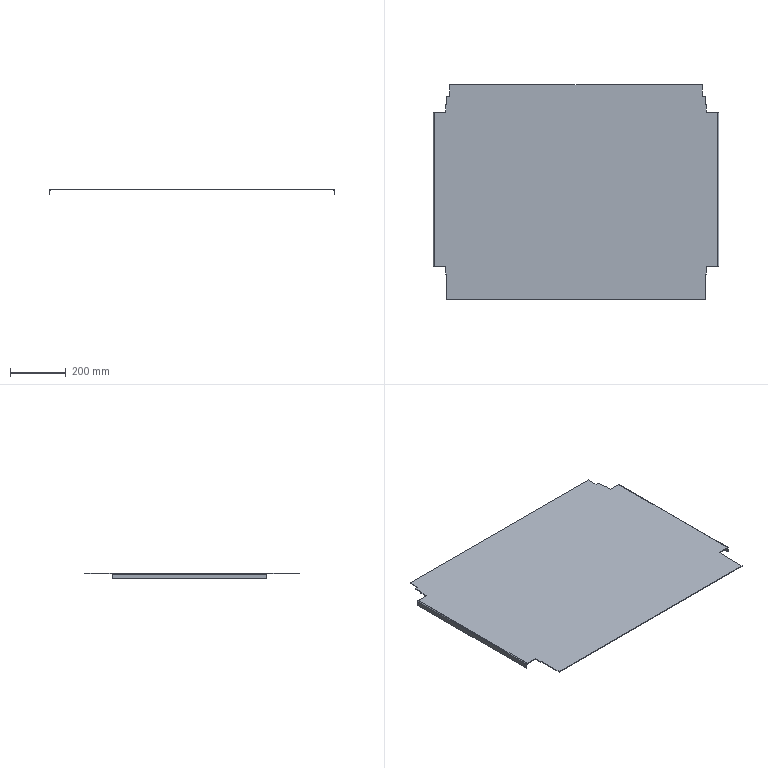Part | SolidWorks | features BaseBody 1 | 1 solid | 42 faces | box 1023 x 767.4 x 20 mm | volume 1955207 mm3 | plane 38 | cylinder 4 | commonest cylinder face diameters 2 x2 7 x2
STEP:
#1=CARTESIAN_POINT('',(509.,285.7,-20.));
#2=VERTEX_POINT('',#1);
#3=CARTESIAN_POINT('',(509.,-266.55,-20.));
#4=VERTEX_POINT('',#3);
#5=CARTESIAN_POINT('',(509.,0.,-20.));
#6=DIRECTION('',(0.,-1.,0.));
#7=VECTOR('',#6,1000.);
#8=LINE('',#5,#7);
#9=EDGE_CURVE('',#2,#4,#8,.T.);
#10=ORIENTED_EDGE('',*,*,#9,.F.);
#11=CARTESIAN_POINT('',(511.5,285.7,-20.));
#12=VERTEX_POINT('',#11);
#13=CARTESIAN_POINT('',(511.5,285.7,-20.));
#14=DIRECTION('',(-1.,0.,0.));
#15=VECTOR('',#14,1000.);
#16=LINE('',#13,#15);
#17=EDGE_CURVE('',#12,#2,#16,.T.);
#18=ORIENTED_EDGE('',*,*,#17,.F.);
#19=CARTESIAN_POINT('',(511.5,-266.55,-20.));
#20=VERTEX_POINT('',#19);
#21=CARTESIAN_POINT('',(511.5,-266.55,-20.));
#22=DIRECTION('',(0.,-1.,0.));
#23=VECTOR('',#22,1000.);
#24=LINE('',#21,#23);
#25=EDGE_CURVE('',#12,#20,#24,.T.);
#26=ORIENTED_EDGE('',*,*,#25,.T.);
#27=CARTESIAN_POINT('',(511.5,-266.55,-20.));
#28=DIRECTION('',(-1.,0.,0.));
#29=VECTOR('',#28,1000.);
#30=LINE('',#27,#29);
#31=EDGE_CURVE('',#20,#4,#30,.T.);
#32=ORIENTED_EDGE('',*,*,#31,.T.);
#33=EDGE_LOOP('',(#10,#18,#26,#32));
#34=FACE_OUTER_BOUND('',#33,.T.);
#35=CARTESIAN_POINT('',(511.5,-266.55,-20.));
#36=DIRECTION('',(0.,0.,-1.));
#37=DIRECTION('',(0.,-1.,0.));
#38=AXIS2_PLACEMENT_3D('',#35,#36,#37);
#39=PLANE('',#38);
#40=ADVANCED_FACE('',(#34),#39,.T.);
#41=CARTESIAN_POINT('',(509.,285.7,-3.5));
#42=VERTEX_POINT('',#41);
#43=CARTESIAN_POINT('',(509.,-266.55,-3.5));
#44=VERTEX_POINT('',#43);
#45=CARTESIAN_POINT('',(509.,285.7,-3.5));
#46=DIRECTION('',(0.,-1.,0.));
#47=VECTOR('',#46,1000.);
#48=LINE('',#45,#47);
#49=EDGE_CURVE('',#42,#44,#48,.T.);
#50=ORIENTED_EDGE('',*,*,#49,.F.);
#51=CARTESIAN_POINT('',(509.,285.7,0.));
#52=DIRECTION('',(0.,0.,-1.));
#53=VECTOR('',#52,1000.);
#54=LINE('',#51,#53);
#55=EDGE_CURVE('',#42,#2,#54,.T.);
#56=ORIENTED_EDGE('',*,*,#55,.T.);
#57=ORIENTED_EDGE('',*,*,#9,.T.);
#58=CARTESIAN_POINT('',(509.,-266.55,0.));
#59=DIRECTION('',(0.,0.,1.));
#60=VECTOR('',#59,1000.);
#61=LINE('',#58,#60);
#62=EDGE_CURVE('',#4,#44,#61,.T.);
#63=ORIENTED_EDGE('',*,*,#62,.T.);
#64=EDGE_LOOP('',(#50,#56,#57,#63));
#65=FACE_OUTER_BOUND('',#64,.T.);
#66=CARTESIAN_POINT('',(509.,0.,0.));
#67=DIRECTION('',(1.,0.,0.));
#68=DIRECTION('',(0.,0.,1.));
#69=AXIS2_PLACEMENT_3D('',#66,#67,#68);
#70=PLANE('',#69);
#71=ADVANCED_FACE('',(#65),#70,.F.);
#72=CARTESIAN_POINT('',(511.5,285.7,-3.5));
#73=VERTEX_POINT('',#72);
#74=CARTESIAN_POINT('',(511.5,285.7,-20.));
#75=DIRECTION('',(0.,0.,-1.));
#76=VECTOR('',#75,1000.);
#77=LINE('',#74,#76);
#78=EDGE_CURVE('',#73,#12,#77,.T.);
#79=ORIENTED_EDGE('',*,*,#78,.F.);
#80=CARTESIAN_POINT('',(511.5,-266.55,-3.5));
#81=VERTEX_POINT('',#80);
#82=CARTESIAN_POINT('',(511.5,0.,-3.5));
#83=DIRECTION('',(0.,-1.,0.));
#84=VECTOR('',#83,1000.);
#85=LINE('',#82,#84);
#86=EDGE_CURVE('',#73,#81,#85,.T.);
#87=ORIENTED_EDGE('',*,*,#86,.T.);
#88=CARTESIAN_POINT('',(511.5,-266.55,-2.5));
#89=DIRECTION('',(0.,0.,1.));
#90=VECTOR('',#89,1000.);
#91=LINE('',#88,#90);
#92=EDGE_CURVE('',#20,#81,#91,.T.);
#93=ORIENTED_EDGE('',*,*,#92,.F.);
#94=ORIENTED_EDGE('',*,*,#25,.F.);
#95=EDGE_LOOP('',(#79,#87,#93,#94));
#96=FACE_OUTER_BOUND('',#95,.T.);
#97=CARTESIAN_POINT('',(511.5,0.,0.));
#98=DIRECTION('',(1.,0.,0.));
#99=DIRECTION('',(0.,0.,1.));
#100=AXIS2_PLACEMENT_3D('',#97,#98,#99);
#101=PLANE('',#100);
#102=ADVANCED_FACE('',(#96),#101,.T.);
#103=ORIENTED_EDGE('',*,*,#55,.F.);
#104=CARTESIAN_POINT('',(511.5,285.7,-3.5));
#105=DIRECTION('',(1.,0.,0.));
#106=VECTOR('',#105,1000.);
#107=LINE('',#104,#106);
#108=EDGE_CURVE('',#42,#73,#107,.T.);
#109=ORIENTED_EDGE('',*,*,#108,.T.);
#110=ORIENTED_EDGE('',*,*,#78,.T.);
#111=ORIENTED_EDGE('',*,*,#17,.T.);
#112=EDGE_LOOP('',(#103,#109,#110,#111));
#113=FACE_OUTER_BOUND('',#112,.T.);
#114=CARTESIAN_POINT('',(511.5,285.7,-20.));
#115=DIRECTION('',(0.,1.,0.));
#116=DIRECTION('',(1.,0.,0.));
#117=AXIS2_PLACEMENT_3D('',#114,#115,#116);
#118=PLANE('',#117);
#119=ADVANCED_FACE('',(#113),#118,.T.);
#120=ORIENTED_EDGE('',*,*,#92,.T.);
#121=CARTESIAN_POINT('',(509.,-266.55,-3.5));
#122=DIRECTION('',(1.,0.,0.));
#123=VECTOR('',#122,1000.);
#124=LINE('',#121,#123);
#125=EDGE_CURVE('',#44,#81,#124,.T.);
#126=ORIENTED_EDGE('',*,*,#125,.F.);
#127=ORIENTED_EDGE('',*,*,#62,.F.);
#128=ORIENTED_EDGE('',*,*,#31,.F.);
#129=EDGE_LOOP('',(#120,#126,#127,#128));
#130=FACE_OUTER_BOUND('',#129,.T.);
#131=CARTESIAN_POINT('',(511.5,-266.55,-2.5));
#132=DIRECTION('',(0.,-1.,0.));
#133=DIRECTION('',(0.,0.,-1.));
#134=AXIS2_PLACEMENT_3D('',#131,#132,#133);
#135=PLANE('',#134);
#136=ADVANCED_FACE('',(#130),#135,.T.);
#137=CARTESIAN_POINT('',(508.,-266.55,-2.5));
#138=VERTEX_POINT('',#137);
#139=CARTESIAN_POINT('',(508.,285.7,-2.5));
#140=VERTEX_POINT('',#139);
#141=CARTESIAN_POINT('',(508.,-266.55,-2.5));
#142=DIRECTION('',(0.,1.,0.));
#143=VECTOR('',#142,1000.);
#144=LINE('',#141,#143);
#145=EDGE_CURVE('',#138,#140,#144,.T.);
#146=ORIENTED_EDGE('',*,*,#145,.T.);
#147=CARTESIAN_POINT('',(508.,285.7,-3.5));
#148=DIRECTION('',(0.,1.,0.));
#149=DIRECTION('',(0.,0.,-1.));
#150=AXIS2_PLACEMENT_3D('',#147,#148,#149);
#151=CIRCLE('',#150,1.);
#152=EDGE_CURVE('',#140,#42,#151,.T.);
#153=ORIENTED_EDGE('',*,*,#152,.T.);
#154=ORIENTED_EDGE('',*,*,#49,.T.);
#155=CARTESIAN_POINT('',(508.,-266.55,-3.5));
#156=DIRECTION('',(0.,-1.,0.));
#157=DIRECTION('',(0.,0.,-1.));
#158=AXIS2_PLACEMENT_3D('',#155,#156,#157);
#159=CIRCLE('',#158,1.);
#160=EDGE_CURVE('',#44,#138,#159,.T.);
#161=ORIENTED_EDGE('',*,*,#160,.T.);
#162=EDGE_LOOP('',(#146,#153,#154,#161));
#163=FACE_OUTER_BOUND('',#162,.T.);
#164=CARTESIAN_POINT('',(508.,-266.55,-3.5));
#165=DIRECTION('',(0.,-1.,0.));
#166=DIRECTION('',(1.,0.,0.));
#167=AXIS2_PLACEMENT_3D('',#164,#165,#166);
#168=CYLINDRICAL_SURFACE('',#167,1.);
#169=ADVANCED_FACE('',(#163),#168,.F.);
#170=CARTESIAN_POINT('',(508.,-266.55,0.));
#171=VERTEX_POINT('',#170);
#172=CARTESIAN_POINT('',(508.,285.7,0.));
#173=VERTEX_POINT('',#172);
#174=CARTESIAN_POINT('',(508.,-266.55,0.));
#175=DIRECTION('',(0.,1.,0.));
#176=VECTOR('',#175,1000.);
#177=LINE('',#174,#176);
#178=EDGE_CURVE('',#171,#173,#177,.T.);
#179=ORIENTED_EDGE('',*,*,#178,.F.);
#180=CARTESIAN_POINT('',(508.,-266.55,-3.5));
#181=DIRECTION('',(0.,-1.,0.));
#182=DIRECTION('',(0.,0.,-1.));
#183=AXIS2_PLACEMENT_3D('',#180,#181,#182);
#184=CIRCLE('',#183,3.5);
#185=EDGE_CURVE('',#81,#171,#184,.T.);
#186=ORIENTED_EDGE('',*,*,#185,.F.);
#187=ORIENTED_EDGE('',*,*,#86,.F.);
#188=CARTESIAN_POINT('',(508.,285.7,-3.5));
#189=DIRECTION('',(0.,1.,0.));
#190=DIRECTION('',(0.,0.,-1.));
#191=AXIS2_PLACEMENT_3D('',#188,#189,#190);
#192=CIRCLE('',#191,3.5);
#193=EDGE_CURVE('',#173,#73,#192,.T.);
#194=ORIENTED_EDGE('',*,*,#193,.F.);
#195=EDGE_LOOP('',(#179,#186,#187,#194));
#196=FACE_OUTER_BOUND('',#195,.T.);
#197=CARTESIAN_POINT('',(508.,-266.55,-3.5));
#198=DIRECTION('',(0.,-1.,0.));
#199=DIRECTION('',(1.,0.,0.));
#200=AXIS2_PLACEMENT_3D('',#197,#198,#199);
#201=CYLINDRICAL_SURFACE('',#200,3.5);
#202=ADVANCED_FACE('',(#196),#201,.T.);
#203=ORIENTED_EDGE('',*,*,#160,.F.);
#204=ORIENTED_EDGE('',*,*,#125,.T.);
#205=ORIENTED_EDGE('',*,*,#185,.T.);
#206=CARTESIAN_POINT('',(508.,-266.55,-2.5));
#207=DIRECTION('',(0.,0.,1.));
#208=VECTOR('',#207,1000.);
#209=LINE('',#206,#208);
#210=EDGE_CURVE('',#138,#171,#209,.T.);
#211=ORIENTED_EDGE('',*,*,#210,.F.);
#212=EDGE_LOOP('',(#203,#204,#205,#211));
#213=FACE_OUTER_BOUND('',#212,.T.);
#214=CARTESIAN_POINT('',(508.,-266.55,-3.5));
#215=DIRECTION('',(0.,1.,0.));
#216=DIRECTION('',(1.,0.,0.));
#217=AXIS2_PLACEMENT_3D('',#214,#215,#216);
#218=PLANE('',#217);
#219=ADVANCED_FACE('',(#213),#218,.F.);
#220=ORIENTED_EDGE('',*,*,#108,.F.);
#221=ORIENTED_EDGE('',*,*,#152,.F.);
#222=CARTESIAN_POINT('',(508.,285.7,-2.5));
#223=DIRECTION('',(0.,0.,1.));
#224=VECTOR('',#223,1000.);
#225=LINE('',#222,#224);
#226=EDGE_CURVE('',#140,#173,#225,.T.);
#227=ORIENTED_EDGE('',*,*,#226,.T.);
#228=ORIENTED_EDGE('',*,*,#193,.T.);
#229=EDGE_LOOP('',(#220,#221,#227,#228));
#230=FACE_OUTER_BOUND('',#229,.T.);
#231=CARTESIAN_POINT('',(508.,285.7,-3.5));
#232=DIRECTION('',(0.,1.,0.));
#233=DIRECTION('',(1.,0.,0.));
#234=AXIS2_PLACEMENT_3D('',#231,#232,#233);
#235=PLANE('',#234);
#236=ADVANCED_FACE('',(#230),#235,.T.);
#237=CARTESIAN_POINT('',(-509.,-266.55,-20.));
#238=VERTEX_POINT('',#237);
#239=CARTESIAN_POINT('',(-509.,285.7,-20.));
#240=VERTEX_POINT('',#239);
#241=CARTESIAN_POINT('',(-509.,0.,-20.));
#242=DIRECTION('',(0.,1.,0.));
#243=VECTOR('',#242,1000.);
#244=LINE('',#241,#243);
#245=EDGE_CURVE('',#238,#240,#244,.T.);
#246=ORIENTED_EDGE('',*,*,#245,.F.);
#247=CARTESIAN_POINT('',(-511.5,-266.55,-20.));
#248=VERTEX_POINT('',#247);
#249=CARTESIAN_POINT('',(-511.5,-266.55,-20.));
#250=DIRECTION('',(1.,0.,0.));
#251=VECTOR('',#250,1000.);
#252=LINE('',#249,#251);
#253=EDGE_CURVE('',#248,#238,#252,.T.);
#254=ORIENTED_EDGE('',*,*,#253,.F.);
#255=CARTESIAN_POINT('',(-511.5,285.7,-20.));
#256=VERTEX_POINT('',#255);
#257=CARTESIAN_POINT('',(-511.5,285.7,-20.));
#258=DIRECTION('',(0.,1.,0.));
#259=VECTOR('',#258,1000.);
#260=LINE('',#257,#259);
#261=EDGE_CURVE('',#248,#256,#260,.T.);
#262=ORIENTED_EDGE('',*,*,#261,.T.);
#263=CARTESIAN_POINT('',(-511.5,285.7,-20.));
#264=DIRECTION('',(1.,0.,0.));
#265=VECTOR('',#264,1000.);
#266=LINE('',#263,#265);
#267=EDGE_CURVE('',#256,#240,#266,.T.);
#268=ORIENTED_EDGE('',*,*,#267,.T.);
#269=EDGE_LOOP('',(#246,#254,#262,#268));
#270=FACE_OUTER_BOUND('',#269,.T.);
#271=CARTESIAN_POINT('',(-511.5,285.7,-20.));
#272=DIRECTION('',(0.,0.,-1.));
#273=DIRECTION('',(-1.,0.,0.));
#274=AXIS2_PLACEMENT_3D('',#271,#272,#273);
#275=PLANE('',#274);
#276=ADVANCED_FACE('',(#270),#275,.T.);
#277=CARTESIAN_POINT('',(-509.,-266.55,-3.5));
#278=VERTEX_POINT('',#277);
#279=CARTESIAN_POINT('',(-509.,285.7,-3.5));
#280=VERTEX_POINT('',#279);
#281=CARTESIAN_POINT('',(-509.,-266.55,-3.5));
#282=DIRECTION('',(0.,1.,0.));
#283=VECTOR('',#282,1000.);
#284=LINE('',#281,#283);
#285=EDGE_CURVE('',#278,#280,#284,.T.);
#286=ORIENTED_EDGE('',*,*,#285,.F.);
#287=CARTESIAN_POINT('',(-509.,-266.55,0.));
#288=DIRECTION('',(0.,0.,-1.));
#289=VECTOR('',#288,1000.);
#290=LINE('',#287,#289);
#291=EDGE_CURVE('',#278,#238,#290,.T.);
#292=ORIENTED_EDGE('',*,*,#291,.T.);
#293=ORIENTED_EDGE('',*,*,#245,.T.);
#294=CARTESIAN_POINT('',(-509.,285.7,0.));
#295=DIRECTION('',(0.,0.,1.));
#296=VECTOR('',#295,1000.);
#297=LINE('',#294,#296);
#298=EDGE_CURVE('',#240,#280,#297,.T.);
#299=ORIENTED_EDGE('',*,*,#298,.T.);
#300=EDGE_LOOP('',(#286,#292,#293,#299));
#301=FACE_OUTER_BOUND('',#300,.T.);
#302=CARTESIAN_POINT('',(-509.,0.,0.));
#303=DIRECTION('',(-1.,0.,0.));
#304=DIRECTION('',(0.,1.,0.));
#305=AXIS2_PLACEMENT_3D('',#302,#303,#304);
#306=PLANE('',#305);
#307=ADVANCED_FACE('',(#301),#306,.F.);
#308=CARTESIAN_POINT('',(-511.5,-266.55,-3.5));
#309=VERTEX_POINT('',#308);
#310=CARTESIAN_POINT('',(-511.5,-266.55,-20.));
#311=DIRECTION('',(0.,0.,-1.));
#312=VECTOR('',#311,1000.);
#313=LINE('',#310,#312);
#314=EDGE_CURVE('',#309,#248,#313,.T.);
#315=ORIENTED_EDGE('',*,*,#314,.F.);
#316=CARTESIAN_POINT('',(-511.5,285.7,-3.5));
#317=VERTEX_POINT('',#316);
#318=CARTESIAN_POINT('',(-511.5,0.,-3.5));
#319=DIRECTION('',(0.,1.,0.));
#320=VECTOR('',#319,1000.);
#321=LINE('',#318,#320);
#322=EDGE_CURVE('',#309,#317,#321,.T.);
#323=ORIENTED_EDGE('',*,*,#322,.T.);
#324=CARTESIAN_POINT('',(-511.5,285.7,-2.5));
#325=DIRECTION('',(0.,0.,1.));
#326=VECTOR('',#325,1000.);
#327=LINE('',#324,#326);
#328=EDGE_CURVE('',#256,#317,#327,.T.);
#329=ORIENTED_EDGE('',*,*,#328,.F.);
#330=ORIENTED_EDGE('',*,*,#261,.F.);
#331=EDGE_LOOP('',(#315,#323,#329,#330));
#332=FACE_OUTER_BOUND('',#331,.T.);
#333=CARTESIAN_POINT('',(-511.5,0.,0.));
#334=DIRECTION('',(-1.,0.,0.));
#335=DIRECTION('',(0.,1.,0.));
#336=AXIS2_PLACEMENT_3D('',#333,#334,#335);
#337=PLANE('',#336);
#338=ADVANCED_FACE('',(#332),#337,.T.);
#339=ORIENTED_EDGE('',*,*,#291,.F.);
#340=CARTESIAN_POINT('',(-511.5,-266.55,-3.5));
#341=DIRECTION('',(-1.,0.,0.));
#342=VECTOR('',#341,1000.);
#343=LINE('',#340,#342);
#344=EDGE_CURVE('',#278,#309,#343,.T.);
#345=ORIENTED_EDGE('',*,*,#344,.T.);
#346=ORIENTED_EDGE('',*,*,#314,.T.);
#347=ORIENTED_EDGE('',*,*,#253,.T.);
#348=EDGE_LOOP('',(#339,#345,#346,#347));
#349=FACE_OUTER_BOUND('',#348,.T.);
#350=CARTESIAN_POINT('',(-511.5,-266.55,-20.));
#351=DIRECTION('',(0.,-1.,0.));
#352=DIRECTION('',(0.,0.,-1.));
#353=AXIS2_PLACEMENT_3D('',#350,#351,#352);
#354=PLANE('',#353);
#355=ADVANCED_FACE('',(#349),#354,.T.);
#356=ORIENTED_EDGE('',*,*,#328,.T.);
#357=CARTESIAN_POINT('',(-509.,285.7,-3.5));
#358=DIRECTION('',(-1.,0.,0.));
#359=VECTOR('',#358,1000.);
#360=LINE('',#357,#359);
#361=EDGE_CURVE('',#280,#317,#360,.T.);
#362=ORIENTED_EDGE('',*,*,#361,.F.);
#363=ORIENTED_EDGE('',*,*,#298,.F.);
#364=ORIENTED_EDGE('',*,*,#267,.F.);
#365=EDGE_LOOP('',(#356,#362,#363,#364));
#366=FACE_OUTER_BOUND('',#365,.T.);
#367=CARTESIAN_POINT('',(-511.5,285.7,-2.5));
#368=DIRECTION('',(0.,1.,0.));
#369=DIRECTION('',(1.,0.,0.));
#370=AXIS2_PLACEMENT_3D('',#367,#368,#369);
#371=PLANE('',#370);
#372=ADVANCED_FACE('',(#366),#371,.T.);
#373=CARTESIAN_POINT('',(-508.,285.7,-2.5));
#374=VERTEX_POINT('',#373);
#375=CARTESIAN_POINT('',(-508.,-266.55,-2.5));
#376=VERTEX_POINT('',#375);
#377=CARTESIAN_POINT('',(-508.,285.7,-2.5));
#378=DIRECTION('',(0.,-1.,0.));
#379=VECTOR('',#378,1000.);
#380=LINE('',#377,#379);
#381=EDGE_CURVE('',#374,#376,#380,.T.);
#382=ORIENTED_EDGE('',*,*,#381,.T.);
#383=CARTESIAN_POINT('',(-508.,-266.55,-3.5));
#384=DIRECTION('',(0.,-1.,0.));
#385=DIRECTION('',(0.,0.,1.));
#386=AXIS2_PLACEMENT_3D('',#383,#384,#385);
#387=CIRCLE('',#386,1.);
#388=EDGE_CURVE('',#376,#278,#387,.T.);
#389=ORIENTED_EDGE('',*,*,#388,.T.);
#390=ORIENTED_EDGE('',*,*,#285,.T.);
#391=CARTESIAN_POINT('',(-508.,285.7,-3.5));
#392=DIRECTION('',(0.,1.,0.));
#393=DIRECTION('',(0.,0.,1.));
#394=AXIS2_PLACEMENT_3D('',#391,#392,#393);
#395=CIRCLE('',#394,1.);
#396=EDGE_CURVE('',#280,#374,#395,.T.);
#397=ORIENTED_EDGE('',*,*,#396,.T.);
#398=EDGE_LOOP('',(#382,#389,#390,#397));
#399=FACE_OUTER_BOUND('',#398,.T.);
#400=CARTESIAN_POINT('',(-508.,285.7,-3.5));
#401=DIRECTION('',(0.,1.,0.));
#402=DIRECTION('',(-1.,0.,0.));
#403=AXIS2_PLACEMENT_3D('',#400,#401,#402);
#404=CYLINDRICAL_SURFACE('',#403,1.);
#405=ADVANCED_FACE('',(#399),#404,.F.);
#406=CARTESIAN_POINT('',(-508.,285.7,0.));
#407=VERTEX_POINT('',#406);
#408=CARTESIAN_POINT('',(-508.,-266.55,0.));
#409=VERTEX_POINT('',#408);
#410=CARTESIAN_POINT('',(-508.,285.7,0.));
#411=DIRECTION('',(0.,-1.,0.));
#412=VECTOR('',#411,1000.);
#413=LINE('',#410,#412);
#414=EDGE_CURVE('',#407,#409,#413,.T.);
#415=ORIENTED_EDGE('',*,*,#414,.F.);
#416=CARTESIAN_POINT('',(-508.,285.7,-3.5));
#417=DIRECTION('',(0.,1.,0.));
#418=DIRECTION('',(0.,0.,1.));
#419=AXIS2_PLACEMENT_3D('',#416,#417,#418);
#420=CIRCLE('',#419,3.5);
#421=EDGE_CURVE('',#317,#407,#420,.T.);
#422=ORIENTED_EDGE('',*,*,#421,.F.);
#423=ORIENTED_EDGE('',*,*,#322,.F.);
#424=CARTESIAN_POINT('',(-508.,-266.55,-3.5));
#425=DIRECTION('',(0.,-1.,0.));
#426=DIRECTION('',(0.,0.,1.));
#427=AXIS2_PLACEMENT_3D('',#424,#425,#426);
#428=CIRCLE('',#427,3.5);
#429=EDGE_CURVE('',#409,#309,#428,.T.);
#430=ORIENTED_EDGE('',*,*,#429,.F.);
#431=EDGE_LOOP('',(#415,#422,#423,#430));
#432=FACE_OUTER_BOUND('',#431,.T.);
#433=CARTESIAN_POINT('',(-508.,285.7,-3.5));
#434=DIRECTION('',(0.,1.,0.));
#435=DIRECTION('',(-1.,0.,0.));
#436=AXIS2_PLACEMENT_3D('',#433,#434,#435);
#437=CYLINDRICAL_SURFACE('',#436,3.5);
#438=ADVANCED_FACE('',(#432),#437,.T.);
#439=ORIENTED_EDGE('',*,*,#396,.F.);
#440=ORIENTED_EDGE('',*,*,#361,.T.);
#441=ORIENTED_EDGE('',*,*,#421,.T.);
#442=CARTESIAN_POINT('',(-508.,285.7,-2.5));
#443=DIRECTION('',(0.,0.,1.));
#444=VECTOR('',#443,1000.);
#445=LINE('',#442,#444);
#446=EDGE_CURVE('',#374,#407,#445,.T.);
#447=ORIENTED_EDGE('',*,*,#446,.F.);
#448=EDGE_LOOP('',(#439,#440,#441,#447));
#449=FACE_OUTER_BOUND('',#448,.T.);
#450=CARTESIAN_POINT('',(-508.,285.7,-3.5));
#451=DIRECTION('',(0.,-1.,0.));
#452=DIRECTION('',(0.,0.,-1.));
#453=AXIS2_PLACEMENT_3D('',#450,#451,#452);
#454=PLANE('',#453);
#455=ADVANCED_FACE('',(#449),#454,.F.);
#456=ORIENTED_EDGE('',*,*,#344,.F.);
#457=ORIENTED_EDGE('',*,*,#388,.F.);
#458=CARTESIAN_POINT('',(-508.,-266.55,-2.5));
#459=DIRECTION('',(0.,0.,1.));
#460=VECTOR('',#459,1000.);
#461=LINE('',#458,#460);
#462=EDGE_CURVE('',#376,#409,#461,.T.);
#463=ORIENTED_EDGE('',*,*,#462,.T.);
#464=ORIENTED_EDGE('',*,*,#429,.T.);
#465=EDGE_LOOP('',(#456,#457,#463,#464));
#466=FACE_OUTER_BOUND('',#465,.T.);
#467=CARTESIAN_POINT('',(-508.,-266.55,-3.5));
#468=DIRECTION('',(0.,-1.,0.));
#469=DIRECTION('',(0.,0.,-1.));
#470=AXIS2_PLACEMENT_3D('',#467,#468,#469);
#471=PLANE('',#470);
#472=ADVANCED_FACE('',(#466),#471,.T.);
#473=CARTESIAN_POINT('',(467.,-266.55,0.));
#474=VERTEX_POINT('',#473);
#475=CARTESIAN_POINT('',(467.,-294.05,0.));
#476=VERTEX_POINT('',#475);
#477=CARTESIAN_POINT('',(467.,-294.05,0.));
#478=DIRECTION('',(0.,-1.,0.));
#479=VECTOR('',#478,1000.);
#480=LINE('',#477,#479);
#481=EDGE_CURVE('',#474,#476,#480,.T.);
#482=ORIENTED_EDGE('',*,*,#481,.T.);
#483=CARTESIAN_POINT('',(467.,-294.05,-2.5));
#484=VERTEX_POINT('',#483);
#485=CARTESIAN_POINT('',(467.,-294.05,-2.5));
#486=DIRECTION('',(0.,0.,1.));
#487=VECTOR('',#486,1000.);
#488=LINE('',#485,#487);
#489=EDGE_CURVE('',#484,#476,#488,.T.);
#490=ORIENTED_EDGE('',*,*,#489,.F.);
#491=CARTESIAN_POINT('',(467.,-266.55,-2.5));
#492=VERTEX_POINT('',#491);
#493=CARTESIAN_POINT('',(467.,-294.05,-2.5));
#494=DIRECTION('',(0.,-1.,0.));
#495=VECTOR('',#494,1000.);
#496=LINE('',#493,#495);
#497=EDGE_CURVE('',#492,#484,#496,.T.);
#498=ORIENTED_EDGE('',*,*,#497,.F.);
#499=CARTESIAN_POINT('',(467.,-266.55,-2.5));
#500=DIRECTION('',(0.,0.,1.));
#501=VECTOR('',#500,1000.);
#502=LINE('',#499,#501);
#503=EDGE_CURVE('',#492,#474,#502,.T.);
#504=ORIENTED_EDGE('',*,*,#503,.T.);
#505=EDGE_LOOP('',(#482,#490,#498,#504));
#506=FACE_OUTER_BOUND('',#505,.T.);
#507=CARTESIAN_POINT('',(467.,-294.05,-2.5));
#508=DIRECTION('',(-1.,0.,0.));
#509=DIRECTION('',(0.,0.,1.));
#510=AXIS2_PLACEMENT_3D('',#507,#508,#509);
#511=PLANE('',#510);
#512=ADVANCED_FACE('',(#506),#511,.F.);
#513=CARTESIAN_POINT('',(-467.,-294.05,0.));
#514=VERTEX_POINT('',#513);
#515=CARTESIAN_POINT('',(-467.,-266.55,0.));
#516=VERTEX_POINT('',#515);
#517=CARTESIAN_POINT('',(-467.,-294.05,0.));
#518=DIRECTION('',(0.,1.,0.));
#519=VECTOR('',#518,1000.);
#520=LINE('',#517,#519);
#521=EDGE_CURVE('',#514,#516,#520,.T.);
#522=ORIENTED_EDGE('',*,*,#521,.T.);
#523=CARTESIAN_POINT('',(-467.,-266.55,-2.5));
#524=VERTEX_POINT('',#523);
#525=CARTESIAN_POINT('',(-467.,-266.55,-2.5));
#526=DIRECTION('',(0.,0.,1.));
#527=VECTOR('',#526,1000.);
#528=LINE('',#525,#527);
#529=EDGE_CURVE('',#524,#516,#528,.T.);
#530=ORIENTED_EDGE('',*,*,#529,.F.);
#531=CARTESIAN_POINT('',(-467.,-294.05,-2.5));
#532=VERTEX_POINT('',#531);
#533=CARTESIAN_POINT('',(-467.,-294.05,-2.5));
#534=DIRECTION('',(0.,1.,0.));
#535=VECTOR('',#534,1000.);
#536=LINE('',#533,#535);
#537=EDGE_CURVE('',#532,#524,#536,.T.);
#538=ORIENTED_EDGE('',*,*,#537,.F.);
#539=CARTESIAN_POINT('',(-467.,-294.05,-2.5));
#540=DIRECTION('',(0.,0.,1.));
#541=VECTOR('',#540,1000.);
#542=LINE('',#539,#541);
#543=EDGE_CURVE('',#532,#514,#542,.T.);
#544=ORIENTED_EDGE('',*,*,#543,.T.);
#545=EDGE_LOOP('',(#522,#530,#538,#544));
#546=FACE_OUTER_BOUND('',#545,.T.);
#547=CARTESIAN_POINT('',(-467.,-294.05,-2.5));
#548=DIRECTION('',(1.,0.,0.));
#549=DIRECTION('',(0.,1.,0.));
#550=AXIS2_PLACEMENT_3D('',#547,#548,#549);
#551=PLANE('',#550);
#552=ADVANCED_FACE('',(#546),#551,.F.);
#553=CARTESIAN_POINT('',(-467.,285.7,0.));
#554=VERTEX_POINT('',#553);
#555=CARTESIAN_POINT('',(-467.,313.2,0.));
#556=VERTEX_POINT('',#555);
#557=CARTESIAN_POINT('',(-467.,313.2,0.));
#558=DIRECTION('',(0.,1.,0.));
#559=VECTOR('',#558,1000.);
#560=LINE('',#557,#559);
#561=EDGE_CURVE('',#554,#556,#560,.T.);
#562=ORIENTED_EDGE('',*,*,#561,.T.);
#563=CARTESIAN_POINT('',(-467.,313.2,-2.5));
#564=VERTEX_POINT('',#563);
#565=CARTESIAN_POINT('',(-467.,313.2,-2.5));
#566=DIRECTION('',(0.,0.,1.));
#567=VECTOR('',#566,1000.);
#568=LINE('',#565,#567);
#569=EDGE_CURVE('',#564,#556,#568,.T.);
#570=ORIENTED_EDGE('',*,*,#569,.F.);
#571=CARTESIAN_POINT('',(-467.,285.7,-2.5));
#572=VERTEX_POINT('',#571);
#573=CARTESIAN_POINT('',(-467.,313.2,-2.5));
#574=DIRECTION('',(0.,1.,0.));
#575=VECTOR('',#574,1000.);
#576=LINE('',#573,#575);
#577=EDGE_CURVE('',#572,#564,#576,.T.);
#578=ORIENTED_EDGE('',*,*,#577,.F.);
#579=CARTESIAN_POINT('',(-467.,285.7,-2.5));
#580=DIRECTION('',(0.,0.,1.));
#581=VECTOR('',#580,1000.);
#582=LINE('',#579,#581);
#583=EDGE_CURVE('',#572,#554,#582,.T.);
#584=ORIENTED_EDGE('',*,*,#583,.T.);
#585=EDGE_LOOP('',(#562,#570,#578,#584));
#586=FACE_OUTER_BOUND('',#585,.T.);
#587=CARTESIAN_POINT('',(-467.,313.2,-2.5));
#588=DIRECTION('',(1.,0.,0.));
#589=DIRECTION('',(0.,1.,0.));
#590=AXIS2_PLACEMENT_3D('',#587,#588,#589);
#591=PLANE('',#590);
#592=ADVANCED_FACE('',(#586),#591,.F.);
#593=CARTESIAN_POINT('',(467.,313.2,0.));
#594=VERTEX_POINT('',#593);
#595=CARTESIAN_POINT('',(467.,285.7,0.));
#596=VERTEX_POINT('',#595);
#597=CARTESIAN_POINT('',(467.,313.2,0.));
#598=DIRECTION('',(0.,-1.,0.));
#599=VECTOR('',#598,1000.);
#600=LINE('',#597,#599);
#601=EDGE_CURVE('',#594,#596,#600,.T.);
#602=ORIENTED_EDGE('',*,*,#601,.T.);
#603=CARTESIAN_POINT('',(467.,285.7,-2.5));
#604=VERTEX_POINT('',#603);
#605=CARTESIAN_POINT('',(467.,285.7,-2.5));
#606=DIRECTION('',(0.,0.,1.));
#607=VECTOR('',#606,1000.);
#608=LINE('',#605,#607);
#609=EDGE_CURVE('',#604,#596,#608,.T.);
#610=ORIENTED_EDGE('',*,*,#609,.F.);
#611=CARTESIAN_POINT('',(467.,313.2,-2.5));
#612=VERTEX_POINT('',#611);
#613=CARTESIAN_POINT('',(467.,313.2,-2.5));
#614=DIRECTION('',(0.,-1.,0.));
#615=VECTOR('',#614,1000.);
#616=LINE('',#613,#615);
#617=EDGE_CURVE('',#612,#604,#616,.T.);
#618=ORIENTED_EDGE('',*,*,#617,.F.);
#619=CARTESIAN_POINT('',(467.,313.2,-2.5));
#620=DIRECTION('',(0.,0.,1.));
#621=VECTOR('',#620,1000.);
#622=LINE('',#619,#621);
#623=EDGE_CURVE('',#612,#594,#622,.T.);
#624=ORIENTED_EDGE('',*,*,#623,.T.);
#625=EDGE_LOOP('',(#602,#610,#618,#624));
#626=FACE_OUTER_BOUND('',#625,.T.);
#627=CARTESIAN_POINT('',(467.,313.2,-2.5));
#628=DIRECTION('',(-1.,0.,0.));
#629=DIRECTION('',(0.,0.,1.));
#630=AXIS2_PLACEMENT_3D('',#627,#628,#629);
#631=PLANE('',#630);
#632=ADVANCED_FACE('',(#626),#631,.F.);
#633=CARTESIAN_POINT('',(463.5,343.7,0.));
#634=VERTEX_POINT('',#633);
#635=CARTESIAN_POINT('',(463.5,313.2,0.));
#636=VERTEX_POINT('',#635);
#637=CARTESIAN_POINT('',(463.5,343.7,0.));
#638=DIRECTION('',(0.,-1.,0.));
#639=VECTOR('',#638,1000.);
#640=LINE('',#637,#639);
#641=EDGE_CURVE('',#634,#636,#640,.T.);
#642=ORIENTED_EDGE('',*,*,#641,.T.);
#643=CARTESIAN_POINT('',(463.5,313.2,-2.5));
#644=VERTEX_POINT('',#643);
#645=CARTESIAN_POINT('',(463.5,313.2,-2.5));
#646=DIRECTION('',(0.,0.,1.));
#647=VECTOR('',#646,1000.);
#648=LINE('',#645,#647);
#649=EDGE_CURVE('',#644,#636,#648,.T.);
#650=ORIENTED_EDGE('',*,*,#649,.F.);
#651=CARTESIAN_POINT('',(463.5,343.7,-2.5));
#652=VERTEX_POINT('',#651);
#653=CARTESIAN_POINT('',(463.5,343.7,-2.5));
#654=DIRECTION('',(0.,-1.,0.));
#655=VECTOR('',#654,1000.);
#656=LINE('',#653,#655);
#657=EDGE_CURVE('',#652,#644,#656,.T.);
#658=ORIENTED_EDGE('',*,*,#657,.F.);
#659=CARTESIAN_POINT('',(463.5,343.7,-2.5));
#660=DIRECTION('',(0.,0.,1.));
#661=VECTOR('',#660,1000.);
#662=LINE('',#659,#661);
#663=EDGE_CURVE('',#652,#634,#662,.T.);
#664=ORIENTED_EDGE('',*,*,#663,.T.);
#665=EDGE_LOOP('',(#642,#650,#658,#664));
#666=FACE_OUTER_BOUND('',#665,.T.);
#667=CARTESIAN_POINT('',(463.5,343.7,-2.5));
#668=DIRECTION('',(-1.,0.,0.));
#669=DIRECTION('',(0.,1.,0.));
#670=AXIS2_PLACEMENT_3D('',#667,#668,#669);
#671=PLANE('',#670);
#672=ADVANCED_FACE('',(#666),#671,.F.);
#673=CARTESIAN_POINT('',(463.5,313.2,0.));
#674=DIRECTION('',(1.,0.,0.));
#675=VECTOR('',#674,1000.);
#676=LINE('',#673,#675);
#677=EDGE_CURVE('',#636,#594,#676,.T.);
#678=ORIENTED_EDGE('',*,*,#677,.T.);
#679=ORIENTED_EDGE('',*,*,#623,.F.);
#680=CARTESIAN_POINT('',(463.5,313.2,-2.5));
#681=DIRECTION('',(1.,0.,0.));
#682=VECTOR('',#681,1000.);
#683=LINE('',#680,#682);
#684=EDGE_CURVE('',#644,#612,#683,.T.);
#685=ORIENTED_EDGE('',*,*,#684,.F.);
#686=ORIENTED_EDGE('',*,*,#649,.T.);
#687=EDGE_LOOP('',(#678,#679,#685,#686));
#688=FACE_OUTER_BOUND('',#687,.T.);
#689=CARTESIAN_POINT('',(463.5,313.2,-2.5));
#690=DIRECTION('',(0.,-1.,0.));
#691=DIRECTION('',(0.,0.,-1.));
#692=AXIS2_PLACEMENT_3D('',#689,#690,#691);
#693=PLANE('',#692);
#694=ADVANCED_FACE('',(#688),#693,.F.);
#695=CARTESIAN_POINT('',(-463.5,313.2,-2.5));
#696=VERTEX_POINT('',#695);
#697=CARTESIAN_POINT('',(-463.5,313.2,-2.5));
#698=DIRECTION('',(1.,0.,0.));
#699=VECTOR('',#698,1000.);
#700=LINE('',#697,#699);
#701=EDGE_CURVE('',#564,#696,#700,.T.);
#702=ORIENTED_EDGE('',*,*,#701,.F.);
#703=ORIENTED_EDGE('',*,*,#569,.T.);
#704=CARTESIAN_POINT('',(-463.5,313.2,0.));
#705=VERTEX_POINT('',#704);
#706=CARTESIAN_POINT('',(-463.5,313.2,0.));
#707=DIRECTION('',(1.,0.,0.));
#708=VECTOR('',#707,1000.);
#709=LINE('',#706,#708);
#710=EDGE_CURVE('',#556,#705,#709,.T.);
#711=ORIENTED_EDGE('',*,*,#710,.T.);
#712=CARTESIAN_POINT('',(-463.5,313.2,-2.5));
#713=DIRECTION('',(0.,0.,1.));
#714=VECTOR('',#713,1000.);
#715=LINE('',#712,#714);
#716=EDGE_CURVE('',#696,#705,#715,.T.);
#717=ORIENTED_EDGE('',*,*,#716,.F.);
#718=EDGE_LOOP('',(#702,#703,#711,#717));
#719=FACE_OUTER_BOUND('',#718,.T.);
#720=CARTESIAN_POINT('',(-463.5,313.2,-2.5));
#721=DIRECTION('',(0.,-1.,0.));
#722=DIRECTION('',(0.,0.,-1.));
#723=AXIS2_PLACEMENT_3D('',#720,#721,#722);
#724=PLANE('',#723);
#725=ADVANCED_FACE('',(#719),#724,.F.);
#726=CARTESIAN_POINT('',(-463.5,343.7,0.));
#727=VERTEX_POINT('',#726);
#728=CARTESIAN_POINT('',(-463.5,343.7,0.));
#729=DIRECTION('',(0.,1.,0.));
#730=VECTOR('',#729,1000.);
#731=LINE('',#728,#730);
#732=EDGE_CURVE('',#705,#727,#731,.T.);
#733=ORIENTED_EDGE('',*,*,#732,.T.);
#734=CARTESIAN_POINT('',(-463.5,343.7,-2.5));
#735=VERTEX_POINT('',#734);
#736=CARTESIAN_POINT('',(-463.5,343.7,-2.5));
#737=DIRECTION('',(0.,0.,1.));
#738=VECTOR('',#737,1000.);
#739=LINE('',#736,#738);
#740=EDGE_CURVE('',#735,#727,#739,.T.);
#741=ORIENTED_EDGE('',*,*,#740,.F.);
#742=CARTESIAN_POINT('',(-463.5,343.7,-2.5));
#743=DIRECTION('',(0.,1.,0.));
#744=VECTOR('',#743,1000.);
#745=LINE('',#742,#744);
#746=EDGE_CURVE('',#696,#735,#745,.T.);
#747=ORIENTED_EDGE('',*,*,#746,.F.);
#748=ORIENTED_EDGE('',*,*,#716,.T.);
#749=EDGE_LOOP('',(#733,#741,#747,#748));
#750=FACE_OUTER_BOUND('',#749,.T.);
#751=CARTESIAN_POINT('',(-463.5,343.7,-2.5));
#752=DIRECTION('',(1.,0.,0.));
#753=DIRECTION('',(0.,-1.,0.));
#754=AXIS2_PLACEMENT_3D('',#751,#752,#753);
#755=PLANE('',#754);
#756=ADVANCED_FACE('',(#750),#755,.F.);
#757=CARTESIAN_POINT('',(-463.5,-383.7,0.));
#758=VERTEX_POINT('',#757);
#759=CARTESIAN_POINT('',(-463.5,-294.05,0.));
#760=VERTEX_POINT('',#759);
#761=CARTESIAN_POINT('',(-463.5,-383.7,0.));
#762=DIRECTION('',(0.,1.,0.));
#763=VECTOR('',#762,1000.);
#764=LINE('',#761,#763);
#765=EDGE_CURVE('',#758,#760,#764,.T.);
#766=ORIENTED_EDGE('',*,*,#765,.T.);
#767=CARTESIAN_POINT('',(-463.5,-294.05,-2.5));
#768=VERTEX_POINT('',#767);
#769=CARTESIAN_POINT('',(-463.5,-294.05,-2.5));
#770=DIRECTION('',(0.,0.,1.));
#771=VECTOR('',#770,1000.);
#772=LINE('',#769,#771);
#773=EDGE_CURVE('',#768,#760,#772,.T.);
#774=ORIENTED_EDGE('',*,*,#773,.F.);
#775=CARTESIAN_POINT('',(-463.5,-383.7,-2.5));
#776=VERTEX_POINT('',#775);
#777=CARTESIAN_POINT('',(-463.5,-383.7,-2.5));
#778=DIRECTION('',(0.,1.,0.));
#779=VECTOR('',#778,1000.);
#780=LINE('',#777,#779);
#781=EDGE_CURVE('',#776,#768,#780,.T.);
#782=ORIENTED_EDGE('',*,*,#781,.F.);
#783=CARTESIAN_POINT('',(-463.5,-383.7,-2.5));
#784=DIRECTION('',(0.,0.,1.));
#785=VECTOR('',#784,1000.);
#786=LINE('',#783,#785);
#787=EDGE_CURVE('',#776,#758,#786,.T.);
#788=ORIENTED_EDGE('',*,*,#787,.T.);
#789=EDGE_LOOP('',(#766,#774,#782,#788));
#790=FACE_OUTER_BOUND('',#789,.T.);
#791=CARTESIAN_POINT('',(-463.5,-383.7,-2.5));
#792=DIRECTION('',(1.,0.,0.));
#793=DIRECTION('',(0.,1.,0.));
#794=AXIS2_PLACEMENT_3D('',#791,#792,#793);
#795=PLANE('',#794);
#796=ADVANCED_FACE('',(#790),#795,.F.);
#797=CARTESIAN_POINT('',(-511.5,-294.05,0.));
#798=DIRECTION('',(-1.,0.,0.));
#799=VECTOR('',#798,1000.);
#800=LINE('',#797,#799);
#801=EDGE_CURVE('',#760,#514,#800,.T.);
#802=ORIENTED_EDGE('',*,*,#801,.T.);
#803=ORIENTED_EDGE('',*,*,#543,.F.);
#804=CARTESIAN_POINT('',(-511.5,-294.05,-2.5));
#805=DIRECTION('',(-1.,0.,0.));
#806=VECTOR('',#805,1000.);
#807=LINE('',#804,#806);
#808=EDGE_CURVE('',#768,#532,#807,.T.);
#809=ORIENTED_EDGE('',*,*,#808,.F.);
#810=ORIENTED_EDGE('',*,*,#773,.T.);
#811=EDGE_LOOP('',(#802,#803,#809,#810));
#812=FACE_OUTER_BOUND('',#811,.T.);
#813=CARTESIAN_POINT('',(-511.5,-294.05,-2.5));
#814=DIRECTION('',(0.,1.,0.));
#815=DIRECTION('',(1.,0.,0.));
#816=AXIS2_PLACEMENT_3D('',#813,#814,#815);
#817=PLANE('',#816);
#818=ADVANCED_FACE('',(#812),#817,.F.);
#819=CARTESIAN_POINT('',(-451.5,343.7,-2.5));
#820=VERTEX_POINT('',#819);
#821=CARTESIAN_POINT('',(-511.5,343.7,-2.5));
#822=DIRECTION('',(1.,0.,0.));
#823=VECTOR('',#822,1000.);
#824=LINE('',#821,#823);
#825=EDGE_CURVE('',#735,#820,#824,.T.);
#826=ORIENTED_EDGE('',*,*,#825,.F.);
#827=ORIENTED_EDGE('',*,*,#740,.T.);
#828=CARTESIAN_POINT('',(-451.5,343.7,0.));
#829=VERTEX_POINT('',#828);
#830=CARTESIAN_POINT('',(-511.5,343.7,0.));
#831=DIRECTION('',(1.,0.,0.));
#832=VECTOR('',#831,1000.);
#833=LINE('',#830,#832);
#834=EDGE_CURVE('',#727,#829,#833,.T.);
#835=ORIENTED_EDGE('',*,*,#834,.T.);
#836=CARTESIAN_POINT('',(-451.5,343.7,-2.5));
#837=DIRECTION('',(0.,0.,1.));
#838=VECTOR('',#837,1000.);
#839=LINE('',#836,#838);
#840=EDGE_CURVE('',#820,#829,#839,.T.);
#841=ORIENTED_EDGE('',*,*,#840,.F.);
#842=EDGE_LOOP('',(#826,#827,#835,#841));
#843=FACE_OUTER_BOUND('',#842,.T.);
#844=CARTESIAN_POINT('',(-511.5,343.7,-2.5));
#845=DIRECTION('',(0.,-1.,0.));
#846=DIRECTION('',(0.,0.,-1.));
#847=AXIS2_PLACEMENT_3D('',#844,#845,#846);
#848=PLANE('',#847);
#849=ADVANCED_FACE('',(#843),#848,.F.);
#850=CARTESIAN_POINT('',(-451.5,383.7,0.));
#851=VERTEX_POINT('',#850);
#852=CARTESIAN_POINT('',(-451.5,383.7,0.));
#853=DIRECTION('',(0.,1.,0.));
#854=VECTOR('',#853,1000.);
#855=LINE('',#852,#854);
#856=EDGE_CURVE('',#829,#851,#855,.T.);
#857=ORIENTED_EDGE('',*,*,#856,.T.);
#858=CARTESIAN_POINT('',(-451.5,383.7,-2.5));
#859=VERTEX_POINT('',#858);
#860=CARTESIAN_POINT('',(-451.5,383.7,-2.5));
#861=DIRECTION('',(0.,0.,1.));
#862=VECTOR('',#861,1000.);
#863=LINE('',#860,#862);
#864=EDGE_CURVE('',#859,#851,#863,.T.);
#865=ORIENTED_EDGE('',*,*,#864,.F.);
#866=CARTESIAN_POINT('',(-451.5,383.7,-2.5));
#867=DIRECTION('',(0.,1.,0.));
#868=VECTOR('',#867,1000.);
#869=LINE('',#866,#868);
#870=EDGE_CURVE('',#820,#859,#869,.T.);
#871=ORIENTED_EDGE('',*,*,#870,.F.);
#872=ORIENTED_EDGE('',*,*,#840,.T.);
#873=EDGE_LOOP('',(#857,#865,#871,#872));
#874=FACE_OUTER_BOUND('',#873,.T.);
#875=CARTESIAN_POINT('',(-451.5,383.7,-2.5));
#876=DIRECTION('',(1.,0.,0.));
#877=DIRECTION('',(0.,1.,0.));
#878=AXIS2_PLACEMENT_3D('',#875,#876,#877);
#879=PLANE('',#878);
#880=ADVANCED_FACE('',(#874),#879,.F.);
#881=CARTESIAN_POINT('',(451.5,383.7,0.));
#882=VERTEX_POINT('',#881);
#883=CARTESIAN_POINT('',(451.5,343.7,0.));
#884=VERTEX_POINT('',#883);
#885=CARTESIAN_POINT('',(451.5,383.7,0.));
#886=DIRECTION('',(0.,-1.,0.));
#887=VECTOR('',#886,1000.);
#888=LINE('',#885,#887);
#889=EDGE_CURVE('',#882,#884,#888,.T.);
#890=ORIENTED_EDGE('',*,*,#889,.T.);
#891=CARTESIAN_POINT('',(451.5,343.7,-2.5));
#892=VERTEX_POINT('',#891);
#893=CARTESIAN_POINT('',(451.5,343.7,-2.5));
#894=DIRECTION('',(0.,0.,1.));
#895=VECTOR('',#894,1000.);
#896=LINE('',#893,#895);
#897=EDGE_CURVE('',#892,#884,#896,.T.);
#898=ORIENTED_EDGE('',*,*,#897,.F.);
#899=CARTESIAN_POINT('',(451.5,383.7,-2.5));
#900=VERTEX_POINT('',#899);
#901=CARTESIAN_POINT('',(451.5,383.7,-2.5));
#902=DIRECTION('',(0.,-1.,0.));
#903=VECTOR('',#902,1000.);
#904=LINE('',#901,#903);
#905=EDGE_CURVE('',#900,#892,#904,.T.);
#906=ORIENTED_EDGE('',*,*,#905,.F.);
#907=CARTESIAN_POINT('',(451.5,383.7,-2.5));
#908=DIRECTION('',(0.,0.,1.));
#909=VECTOR('',#908,1000.);
#910=LINE('',#907,#909);
#911=EDGE_CURVE('',#900,#882,#910,.T.);
#912=ORIENTED_EDGE('',*,*,#911,.T.);
#913=EDGE_LOOP('',(#890,#898,#906,#912));
#914=FACE_OUTER_BOUND('',#913,.T.);
#915=CARTESIAN_POINT('',(451.5,383.7,-2.5));
#916=DIRECTION('',(-1.,0.,0.));
#917=DIRECTION('',(0.,0.,1.));
#918=AXIS2_PLACEMENT_3D('',#915,#916,#917);
#919=PLANE('',#918);
#920=ADVANCED_FACE('',(#914),#919,.F.);
#921=CARTESIAN_POINT('',(511.5,343.7,0.));
#922=DIRECTION('',(1.,0.,0.));
#923=VECTOR('',#922,1000.);
#924=LINE('',#921,#923);
#925=EDGE_CURVE('',#884,#634,#924,.T.);
#926=ORIENTED_EDGE('',*,*,#925,.T.);
#927=ORIENTED_EDGE('',*,*,#663,.F.);
#928=CARTESIAN_POINT('',(511.5,343.7,-2.5));
#929=DIRECTION('',(1.,0.,0.));
#930=VECTOR('',#929,1000.);
#931=LINE('',#928,#930);
#932=EDGE_CURVE('',#892,#652,#931,.T.);
#933=ORIENTED_EDGE('',*,*,#932,.F.);
#934=ORIENTED_EDGE('',*,*,#897,.T.);
#935=EDGE_LOOP('',(#926,#927,#933,#934));
#936=FACE_OUTER_BOUND('',#935,.T.);
#937=CARTESIAN_POINT('',(511.5,343.7,-2.5));
#938=DIRECTION('',(0.,-1.,0.));
#939=DIRECTION('',(-1.,0.,0.));
#940=AXIS2_PLACEMENT_3D('',#937,#938,#939);
#941=PLANE('',#940);
#942=ADVANCED_FACE('',(#936),#941,.F.);
#943=CARTESIAN_POINT('',(463.5,-294.05,-2.5));
#944=VERTEX_POINT('',#943);
#945=CARTESIAN_POINT('',(511.5,-294.05,-2.5));
#946=DIRECTION('',(-1.,0.,0.));
#947=VECTOR('',#946,1000.);
#948=LINE('',#945,#947);
#949=EDGE_CURVE('',#484,#944,#948,.T.);
#950=ORIENTED_EDGE('',*,*,#949,.F.);
#951=ORIENTED_EDGE('',*,*,#489,.T.);
#952=CARTESIAN_POINT('',(463.5,-294.05,0.));
#953=VERTEX_POINT('',#952);
#954=CARTESIAN_POINT('',(511.5,-294.05,0.));
#955=DIRECTION('',(-1.,0.,0.));
#956=VECTOR('',#955,1000.);
#957=LINE('',#954,#956);
#958=EDGE_CURVE('',#476,#953,#957,.T.);
#959=ORIENTED_EDGE('',*,*,#958,.T.);
#960=CARTESIAN_POINT('',(463.5,-294.05,-2.5));
#961=DIRECTION('',(0.,0.,1.));
#962=VECTOR('',#961,1000.);
#963=LINE('',#960,#962);
#964=EDGE_CURVE('',#944,#953,#963,.T.);
#965=ORIENTED_EDGE('',*,*,#964,.F.);
#966=EDGE_LOOP('',(#950,#951,#959,#965));
#967=FACE_OUTER_BOUND('',#966,.T.);
#968=CARTESIAN_POINT('',(511.5,-294.05,-2.5));
#969=DIRECTION('',(0.,1.,0.));
#970=DIRECTION('',(1.,0.,0.));
#971=AXIS2_PLACEMENT_3D('',#968,#969,#970);
#972=PLANE('',#971);
#973=ADVANCED_FACE('',(#967),#972,.F.);
#974=CARTESIAN_POINT('',(463.5,-383.7,0.));
#975=VERTEX_POINT('',#974);
#976=CARTESIAN_POINT('',(463.5,-383.7,0.));
#977=DIRECTION('',(0.,-1.,0.));
#978=VECTOR('',#977,1000.);
#979=LINE('',#976,#978);
#980=EDGE_CURVE('',#953,#975,#979,.T.);
#981=ORIENTED_EDGE('',*,*,#980,.T.);
#982=CARTESIAN_POINT('',(463.5,-383.7,-2.5));
#983=VERTEX_POINT('',#982);
#984=CARTESIAN_POINT('',(463.5,-383.7,-2.5));
#985=DIRECTION('',(0.,0.,1.));
#986=VECTOR('',#985,1000.);
#987=LINE('',#984,#986);
#988=EDGE_CURVE('',#983,#975,#987,.T.);
#989=ORIENTED_EDGE('',*,*,#988,.F.);
#990=CARTESIAN_POINT('',(463.5,-383.7,-2.5));
#991=DIRECTION('',(0.,-1.,0.));
#992=VECTOR('',#991,1000.);
#993=LINE('',#990,#992);
#994=EDGE_CURVE('',#944,#983,#993,.T.);
#995=ORIENTED_EDGE('',*,*,#994,.F.);
#996=ORIENTED_EDGE('',*,*,#964,.T.);
#997=EDGE_LOOP('',(#981,#989,#995,#996));
#998=FACE_OUTER_BOUND('',#997,.T.);
#999=CARTESIAN_POINT('',(463.5,-383.7,-2.5));
#1000=DIRECTION('',(-1.,0.,0.));
#1001=DIRECTION('',(0.,0.,1.));
#1002=AXIS2_PLACEMENT_3D('',#999,#1000,#1001);
#1003=PLANE('',#1002);
#1004=ADVANCED_FACE('',(#998),#1003,.F.);
#1005=ORIENTED_EDGE('',*,*,#787,.F.);
#1006=CARTESIAN_POINT('',(511.5,-383.7,-2.5));
#1007=DIRECTION('',(1.,0.,0.));
#1008=VECTOR('',#1007,1000.);
#1009=LINE('',#1006,#1008);
#1010=EDGE_CURVE('',#776,#983,#1009,.T.);
#1011=ORIENTED_EDGE('',*,*,#1010,.T.);
#1012=ORIENTED_EDGE('',*,*,#988,.T.);
#1013=CARTESIAN_POINT('',(511.5,-383.7,0.));
#1014=DIRECTION('',(1.,0.,0.));
#1015=VECTOR('',#1014,1000.);
#1016=LINE('',#1013,#1015);
#1017=EDGE_CURVE('',#758,#975,#1016,.T.);
#1018=ORIENTED_EDGE('',*,*,#1017,.F.);
#1019=EDGE_LOOP('',(#1005,#1011,#1012,#1018));
#1020=FACE_OUTER_BOUND('',#1019,.T.);
#1021=CARTESIAN_POINT('',(511.5,-383.7,-2.5));
#1022=DIRECTION('',(0.,-1.,0.));
#1023=DIRECTION('',(0.,0.,-1.));
#1024=AXIS2_PLACEMENT_3D('',#1021,#1022,#1023);
#1025=PLANE('',#1024);
#1026=ADVANCED_FACE('',(#1020),#1025,.T.);
#1027=ORIENTED_EDGE('',*,*,#864,.T.);
#1028=CARTESIAN_POINT('',(511.5,383.7,0.));
#1029=DIRECTION('',(-1.,0.,0.));
#1030=VECTOR('',#1029,1000.);
#1031=LINE('',#1028,#1030);
#1032=EDGE_CURVE('',#882,#851,#1031,.T.);
#1033=ORIENTED_EDGE('',*,*,#1032,.F.);
#1034=ORIENTED_EDGE('',*,*,#911,.F.);
#1035=CARTESIAN_POINT('',(511.5,383.7,-2.5));
#1036=DIRECTION('',(-1.,0.,0.));
#1037=VECTOR('',#1036,1000.);
#1038=LINE('',#1035,#1037);
#1039=EDGE_CURVE('',#900,#859,#1038,.T.);
#1040=ORIENTED_EDGE('',*,*,#1039,.T.);
#1041=EDGE_LOOP('',(#1027,#1033,#1034,#1040));
#1042=FACE_OUTER_BOUND('',#1041,.T.);
#1043=CARTESIAN_POINT('',(511.5,383.7,-2.5));
#1044=DIRECTION('',(0.,1.,0.));
#1045=DIRECTION('',(1.,0.,0.));
#1046=AXIS2_PLACEMENT_3D('',#1043,#1044,#1045);
#1047=PLANE('',#1046);
#1048=ADVANCED_FACE('',(#1042),#1047,.T.);
#1049=ORIENTED_EDGE('',*,*,#462,.F.);
#1050=CARTESIAN_POINT('',(-511.5,-266.55,-2.5));
#1051=DIRECTION('',(-1.,0.,0.));
#1052=VECTOR('',#1051,1000.);
#1053=LINE('',#1050,#1052);
#1054=EDGE_CURVE('',#524,#376,#1053,.T.);
#1055=ORIENTED_EDGE('',*,*,#1054,.F.);
#1056=ORIENTED_EDGE('',*,*,#529,.T.);
#1057=CARTESIAN_POINT('',(-511.5,-266.55,0.));
#1058=DIRECTION('',(-1.,0.,0.));
#1059=VECTOR('',#1058,1000.);
#1060=LINE('',#1057,#1059);
#1061=EDGE_CURVE('',#516,#409,#1060,.T.);
#1062=ORIENTED_EDGE('',*,*,#1061,.T.);
#1063=EDGE_LOOP('',(#1049,#1055,#1056,#1062));
#1064=FACE_OUTER_BOUND('',#1063,.T.);
#1065=CARTESIAN_POINT('',(-511.5,-266.55,-2.5));
#1066=DIRECTION('',(0.,1.,0.));
#1067=DIRECTION('',(1.,0.,0.));
#1068=AXIS2_PLACEMENT_3D('',#1065,#1066,#1067);
#1069=PLANE('',#1068);
#1070=ADVANCED_FACE('',(#1064),#1069,.F.);
#1071=ORIENTED_EDGE('',*,*,#446,.T.);
#1072=CARTESIAN_POINT('',(-511.5,285.7,0.));
#1073=DIRECTION('',(1.,0.,0.));
#1074=VECTOR('',#1073,1000.);
#1075=LINE('',#1072,#1074);
#1076=EDGE_CURVE('',#407,#554,#1075,.T.);
#1077=ORIENTED_EDGE('',*,*,#1076,.T.);
#1078=ORIENTED_EDGE('',*,*,#583,.F.);
#1079=CARTESIAN_POINT('',(-511.5,285.7,-2.5));
#1080=DIRECTION('',(1.,0.,0.));
#1081=VECTOR('',#1080,1000.);
#1082=LINE('',#1079,#1081);
#1083=EDGE_CURVE('',#374,#572,#1082,.T.);
#1084=ORIENTED_EDGE('',*,*,#1083,.F.);
#1085=EDGE_LOOP('',(#1071,#1077,#1078,#1084));
#1086=FACE_OUTER_BOUND('',#1085,.T.);
#1087=CARTESIAN_POINT('',(-511.5,285.7,-2.5));
#1088=DIRECTION('',(0.,-1.,0.));
#1089=DIRECTION('',(0.,0.,-1.));
#1090=AXIS2_PLACEMENT_3D('',#1087,#1088,#1089);
#1091=PLANE('',#1090);
#1092=ADVANCED_FACE('',(#1086),#1091,.F.);
#1093=ORIENTED_EDGE('',*,*,#210,.T.);
#1094=CARTESIAN_POINT('',(511.5,-266.55,0.));
#1095=DIRECTION('',(-1.,0.,0.));
#1096=VECTOR('',#1095,1000.);
#1097=LINE('',#1094,#1096);
#1098=EDGE_CURVE('',#171,#474,#1097,.T.);
#1099=ORIENTED_EDGE('',*,*,#1098,.T.);
#1100=ORIENTED_EDGE('',*,*,#503,.F.);
#1101=CARTESIAN_POINT('',(511.5,-266.55,-2.5));
#1102=DIRECTION('',(-1.,0.,0.));
#1103=VECTOR('',#1102,1000.);
#1104=LINE('',#1101,#1103);
#1105=EDGE_CURVE('',#138,#492,#1104,.T.);
#1106=ORIENTED_EDGE('',*,*,#1105,.F.);
#1107=EDGE_LOOP('',(#1093,#1099,#1100,#1106));
#1108=FACE_OUTER_BOUND('',#1107,.T.);
#1109=CARTESIAN_POINT('',(511.5,-266.55,-2.5));
#1110=DIRECTION('',(0.,1.,0.));
#1111=DIRECTION('',(1.,0.,0.));
#1112=AXIS2_PLACEMENT_3D('',#1109,#1110,#1111);
#1113=PLANE('',#1112);
#1114=ADVANCED_FACE('',(#1108),#1113,.F.);
#1115=ORIENTED_EDGE('',*,*,#226,.F.);
#1116=CARTESIAN_POINT('',(511.5,285.7,-2.5));
#1117=DIRECTION('',(1.,0.,0.));
#1118=VECTOR('',#1117,1000.);
#1119=LINE('',#1116,#1118);
#1120=EDGE_CURVE('',#604,#140,#1119,.T.);
#1121=ORIENTED_EDGE('',*,*,#1120,.F.);
#1122=ORIENTED_EDGE('',*,*,#609,.T.);
#1123=CARTESIAN_POINT('',(511.5,285.7,0.));
#1124=DIRECTION('',(1.,0.,0.));
#1125=VECTOR('',#1124,1000.);
#1126=LINE('',#1123,#1125);
#1127=EDGE_CURVE('',#596,#173,#1126,.T.);
#1128=ORIENTED_EDGE('',*,*,#1127,.T.);
#1129=EDGE_LOOP('',(#1115,#1121,#1122,#1128));
#1130=FACE_OUTER_BOUND('',#1129,.T.);
#1131=CARTESIAN_POINT('',(511.5,285.7,-2.5));
#1132=DIRECTION('',(0.,-1.,0.));
#1133=DIRECTION('',(0.,0.,-1.));
#1134=AXIS2_PLACEMENT_3D('',#1131,#1132,#1133);
#1135=PLANE('',#1134);
#1136=ADVANCED_FACE('',(#1130),#1135,.F.);
#1137=ORIENTED_EDGE('',*,*,#178,.T.);
#1138=ORIENTED_EDGE('',*,*,#1127,.F.);
#1139=ORIENTED_EDGE('',*,*,#601,.F.);
#1140=ORIENTED_EDGE('',*,*,#677,.F.);
#1141=ORIENTED_EDGE('',*,*,#641,.F.);
#1142=ORIENTED_EDGE('',*,*,#925,.F.);
#1143=ORIENTED_EDGE('',*,*,#889,.F.);
#1144=ORIENTED_EDGE('',*,*,#1032,.T.);
#1145=ORIENTED_EDGE('',*,*,#856,.F.);
#1146=ORIENTED_EDGE('',*,*,#834,.F.);
#1147=ORIENTED_EDGE('',*,*,#732,.F.);
#1148=ORIENTED_EDGE('',*,*,#710,.F.);
#1149=ORIENTED_EDGE('',*,*,#561,.F.);
#1150=ORIENTED_EDGE('',*,*,#1076,.F.);
#1151=ORIENTED_EDGE('',*,*,#414,.T.);
#1152=ORIENTED_EDGE('',*,*,#1061,.F.);
#1153=ORIENTED_EDGE('',*,*,#521,.F.);
#1154=ORIENTED_EDGE('',*,*,#801,.F.);
#1155=ORIENTED_EDGE('',*,*,#765,.F.);
#1156=ORIENTED_EDGE('',*,*,#1017,.T.);
#1157=ORIENTED_EDGE('',*,*,#980,.F.);
#1158=ORIENTED_EDGE('',*,*,#958,.F.);
#1159=ORIENTED_EDGE('',*,*,#481,.F.);
#1160=ORIENTED_EDGE('',*,*,#1098,.F.);
#1161=EDGE_LOOP('',(#1137,#1138,#1139,#1140,#1141,#1142,#1143,#1144,#1145,#1146,#1147,#1148,#1149,#1150,#1151,#1152,#1153,#1154,#1155,#1156,#1157,#1158,#1159,#1160));
#1162=FACE_OUTER_BOUND('',#1161,.T.);
#1163=CARTESIAN_POINT('',(0.,0.,0.));
#1164=DIRECTION('',(0.,0.,-1.));
#1165=DIRECTION('',(0.,-1.,0.));
#1166=AXIS2_PLACEMENT_3D('',#1163,#1164,#1165);
#1167=PLANE('',#1166);
#1168=ADVANCED_FACE('',(#1162),#1167,.F.);
#1169=ORIENTED_EDGE('',*,*,#1120,.T.);
#1170=ORIENTED_EDGE('',*,*,#145,.F.);
#1171=ORIENTED_EDGE('',*,*,#1105,.T.);
#1172=ORIENTED_EDGE('',*,*,#497,.T.);
#1173=ORIENTED_EDGE('',*,*,#949,.T.);
#1174=ORIENTED_EDGE('',*,*,#994,.T.);
#1175=ORIENTED_EDGE('',*,*,#1010,.F.);
#1176=ORIENTED_EDGE('',*,*,#781,.T.);
#1177=ORIENTED_EDGE('',*,*,#808,.T.);
#1178=ORIENTED_EDGE('',*,*,#537,.T.);
#1179=ORIENTED_EDGE('',*,*,#1054,.T.);
#1180=ORIENTED_EDGE('',*,*,#381,.F.);
#1181=ORIENTED_EDGE('',*,*,#1083,.T.);
#1182=ORIENTED_EDGE('',*,*,#577,.T.);
#1183=ORIENTED_EDGE('',*,*,#701,.T.);
#1184=ORIENTED_EDGE('',*,*,#746,.T.);
#1185=ORIENTED_EDGE('',*,*,#825,.T.);
#1186=ORIENTED_EDGE('',*,*,#870,.T.);
#1187=ORIENTED_EDGE('',*,*,#1039,.F.);
#1188=ORIENTED_EDGE('',*,*,#905,.T.);
#1189=ORIENTED_EDGE('',*,*,#932,.T.);
#1190=ORIENTED_EDGE('',*,*,#657,.T.);
#1191=ORIENTED_EDGE('',*,*,#684,.T.);
#1192=ORIENTED_EDGE('',*,*,#617,.T.);
#1193=EDGE_LOOP('',(#1169,#1170,#1171,#1172,#1173,#1174,#1175,#1176,#1177,#1178,#1179,#1180,#1181,#1182,#1183,#1184,#1185,#1186,#1187,#1188,#1189,#1190,#1191,#1192));
#1194=FACE_OUTER_BOUND('',#1193,.T.);
#1195=CARTESIAN_POINT('',(0.,0.,-2.5));
#1196=DIRECTION('',(0.,0.,-1.));
#1197=DIRECTION('',(0.,-1.,0.));
#1198=AXIS2_PLACEMENT_3D('',#1195,#1196,#1197);
#1199=PLANE('',#1198);
#1200=ADVANCED_FACE('',(#1194),#1199,.T.);
#1201=CLOSED_SHELL('',(#40,#71,#102,#119,#136,#169,#202,#219,#236,#276,#307,#338,#355,#372,#405,#438,#455,#472,#512,#552,#592,#632,#672,#694,#725,#756,#796,#818,#849,#880,#920,#942,#973,#1004,#1026,#1048,#1070,#1092,#1114,#1136,#1168,#1200));
#1202=MANIFOLD_SOLID_BREP('',#1201);
#1203=CARTESIAN_POINT('',(0.,0.,0.));
#1204=DIRECTION('',(0.,0.,1.));
#1205=DIRECTION('',(1.,0.,0.));
#1206=AXIS2_PLACEMENT_3D('',#1203,#1204,#1205);
#1207=(LENGTH_UNIT()NAMED_UNIT(*)SI_UNIT(.MILLI.,.METRE.));
#1208=UNCERTAINTY_MEASURE_WITH_UNIT(LENGTH_MEASURE(0.00001),#1207,'','');
#1209=(NAMED_UNIT(*)PLANE_ANGLE_UNIT()SI_UNIT($,.RADIAN.));
#1210=(NAMED_UNIT(*)SI_UNIT($,.STERADIAN.)SOLID_ANGLE_UNIT());
#1211=(GEOMETRIC_REPRESENTATION_CONTEXT(3)GLOBAL_UNCERTAINTY_ASSIGNED_CONTEXT((#1208))GLOBAL_UNIT_ASSIGNED_CONTEXT((#1207,#1209,#1210))REPRESENTATION_CONTEXT('',''));
#1212=ADVANCED_BREP_SHAPE_REPRESENTATION('',(#1202,#1206),#1211);